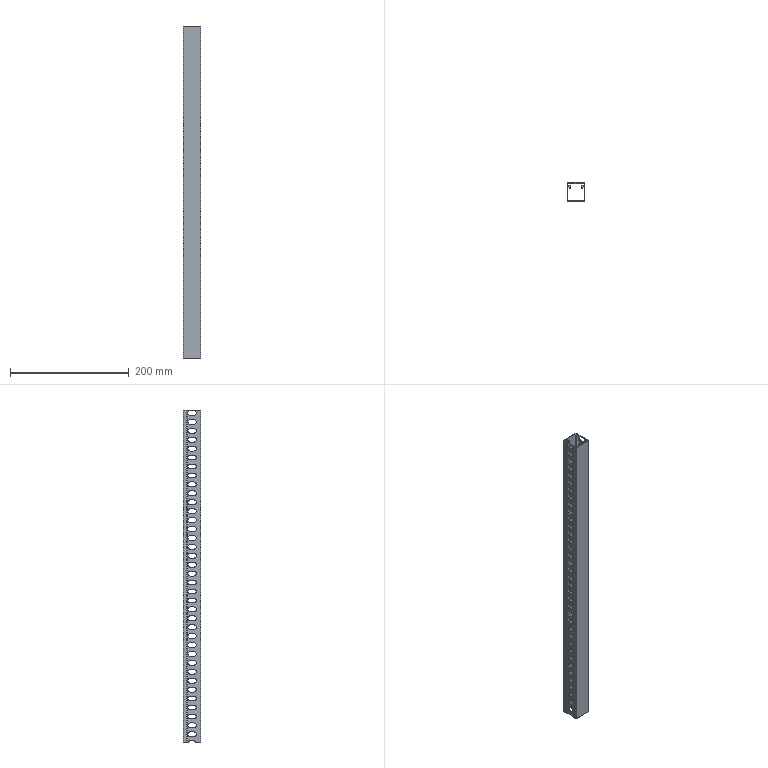Part | SolidWorks | features BaseBody 1 | 1 solid | 329 faces | box 30 x 30 x 558 mm | volume 68573 mm3 | plane 177 | cylinder 152 | commonest cylinder face diameters 8 x152